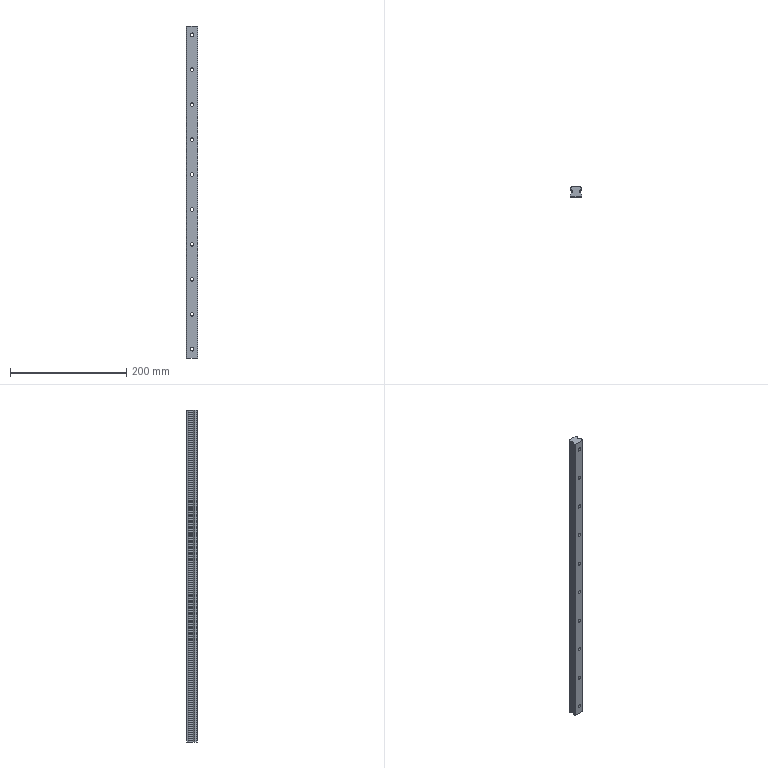Part | SolidWorks | features ICE 2, BaseBody 1, HoleWzd 1, LPattern 1 | 1 solid | 94 faces | box 20 x 17.5 x 570 mm | volume 161806 mm3 | cylinder 62 | plane 32 | commonest cylinder face diameters 6 x20 9.5 x20 1 x12 2 x6 4.06 x4